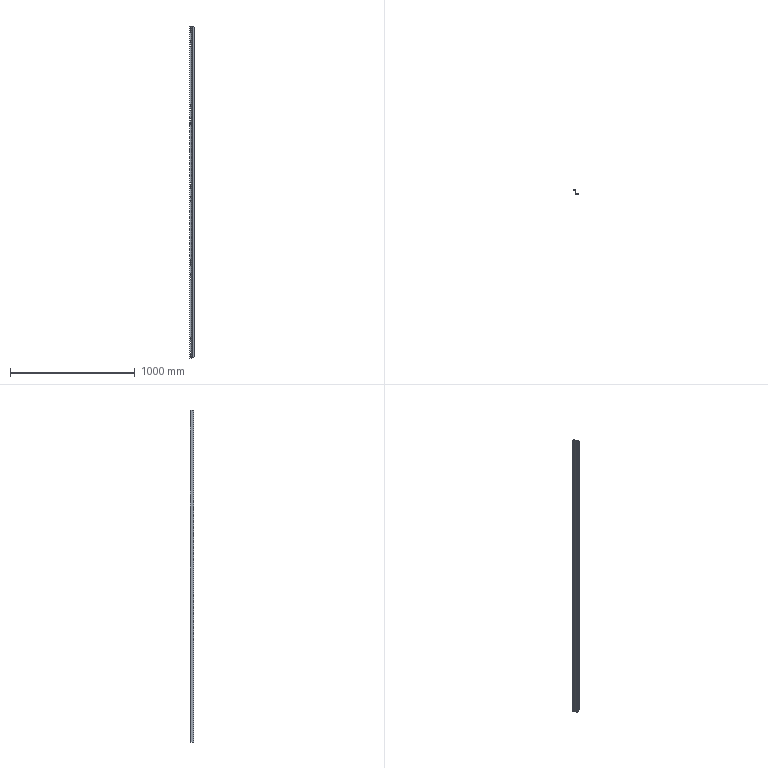Part | STEP file | SK5 | 1 solid | 90 faces | box 38 x 31.5 x 2660 mm | volume 335418 mm3 | plane 46 | cylinder 44 | commonest cylinder face diameters 8.2 x38 6 x2 10 x2 40 x2